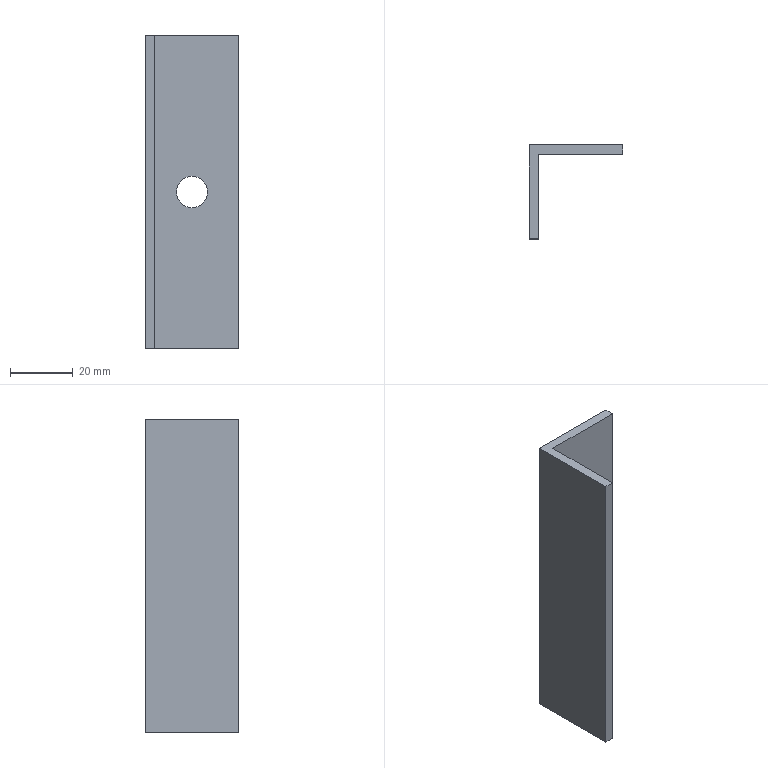Part | SolidWorks | features Extrusion 1, ICE 1 | 1 solid | 10 faces | box 30 x 30 x 100 mm | volume 16864 mm3 | plane 8 | cylinder 2 | commonest cylinder face diameters 10 x2
STEP:
#1=CARTESIAN_POINT('',(15.,-3.,45.));
#2=VERTEX_POINT('',#1);
#3=CARTESIAN_POINT('',(15.,-3.,55.));
#4=VERTEX_POINT('',#3);
#5=CARTESIAN_POINT('',(15.,-3.,50.));
#6=DIRECTION('',(0.,1.,0.));
#7=DIRECTION('',(0.,0.,1.));
#8=AXIS2_PLACEMENT_3D('',#5,#6,#7);
#9=CIRCLE('',#8,5.);
#10=EDGE_CURVE('',#2,#4,#9,.T.);
#11=ORIENTED_EDGE('',*,*,#10,.F.);
#12=CARTESIAN_POINT('',(15.,0.,45.));
#13=VERTEX_POINT('',#12);
#14=CARTESIAN_POINT('',(15.,-10.,45.));
#15=DIRECTION('',(0.,1.,0.));
#16=VECTOR('',#15,1000.);
#17=LINE('',#14,#16);
#18=EDGE_CURVE('',#2,#13,#17,.T.);
#19=ORIENTED_EDGE('',*,*,#18,.T.);
#20=CARTESIAN_POINT('',(15.,0.,55.));
#21=VERTEX_POINT('',#20);
#22=CARTESIAN_POINT('',(15.,0.,50.));
#23=DIRECTION('',(0.,1.,0.));
#24=DIRECTION('',(0.,0.,1.));
#25=AXIS2_PLACEMENT_3D('',#22,#23,#24);
#26=CIRCLE('',#25,5.);
#27=EDGE_CURVE('',#13,#21,#26,.T.);
#28=ORIENTED_EDGE('',*,*,#27,.T.);
#29=CARTESIAN_POINT('',(15.,-10.,55.));
#30=DIRECTION('',(0.,1.,0.));
#31=VECTOR('',#30,1000.);
#32=LINE('',#29,#31);
#33=EDGE_CURVE('',#4,#21,#32,.T.);
#34=ORIENTED_EDGE('',*,*,#33,.F.);
#35=EDGE_LOOP('',(#11,#19,#28,#34));
#36=FACE_OUTER_BOUND('',#35,.T.);
#37=CARTESIAN_POINT('',(15.,-10.,50.));
#38=DIRECTION('',(0.,1.,0.));
#39=DIRECTION('',(0.,0.,1.));
#40=AXIS2_PLACEMENT_3D('',#37,#38,#39);
#41=CYLINDRICAL_SURFACE('',#40,5.);
#42=ADVANCED_FACE('',(#36),#41,.F.);
#43=CARTESIAN_POINT('',(0.,0.,0.));
#44=VERTEX_POINT('',#43);
#45=CARTESIAN_POINT('',(0.,-30.,0.));
#46=VERTEX_POINT('',#45);
#47=CARTESIAN_POINT('',(0.,0.,0.));
#48=DIRECTION('',(0.,-1.,0.));
#49=VECTOR('',#48,1000.);
#50=LINE('',#47,#49);
#51=EDGE_CURVE('',#44,#46,#50,.T.);
#52=ORIENTED_EDGE('',*,*,#51,.T.);
#53=CARTESIAN_POINT('',(0.,-30.,100.));
#54=VERTEX_POINT('',#53);
#55=CARTESIAN_POINT('',(0.,-30.,100.));
#56=DIRECTION('',(0.,0.,-1.));
#57=VECTOR('',#56,1000.);
#58=LINE('',#55,#57);
#59=EDGE_CURVE('',#54,#46,#58,.T.);
#60=ORIENTED_EDGE('',*,*,#59,.F.);
#61=CARTESIAN_POINT('',(0.,0.,100.));
#62=VERTEX_POINT('',#61);
#63=CARTESIAN_POINT('',(0.,0.,100.));
#64=DIRECTION('',(0.,-1.,0.));
#65=VECTOR('',#64,1000.);
#66=LINE('',#63,#65);
#67=EDGE_CURVE('',#62,#54,#66,.T.);
#68=ORIENTED_EDGE('',*,*,#67,.F.);
#69=CARTESIAN_POINT('',(0.,0.,100.));
#70=DIRECTION('',(0.,0.,-1.));
#71=VECTOR('',#70,1000.);
#72=LINE('',#69,#71);
#73=EDGE_CURVE('',#62,#44,#72,.T.);
#74=ORIENTED_EDGE('',*,*,#73,.T.);
#75=EDGE_LOOP('',(#52,#60,#68,#74));
#76=FACE_OUTER_BOUND('',#75,.T.);
#77=CARTESIAN_POINT('',(0.,0.,100.));
#78=DIRECTION('',(1.,0.,0.));
#79=DIRECTION('',(0.,1.,0.));
#80=AXIS2_PLACEMENT_3D('',#77,#78,#79);
#81=PLANE('',#80);
#82=ADVANCED_FACE('',(#76),#81,.F.);
#83=CARTESIAN_POINT('',(3.,-30.,0.));
#84=VERTEX_POINT('',#83);
#85=CARTESIAN_POINT('',(0.,-30.,0.));
#86=DIRECTION('',(1.,0.,0.));
#87=VECTOR('',#86,1000.);
#88=LINE('',#85,#87);
#89=EDGE_CURVE('',#46,#84,#88,.T.);
#90=ORIENTED_EDGE('',*,*,#89,.T.);
#91=CARTESIAN_POINT('',(3.,-30.,100.));
#92=VERTEX_POINT('',#91);
#93=CARTESIAN_POINT('',(3.,-30.,100.));
#94=DIRECTION('',(0.,0.,-1.));
#95=VECTOR('',#94,1000.);
#96=LINE('',#93,#95);
#97=EDGE_CURVE('',#92,#84,#96,.T.);
#98=ORIENTED_EDGE('',*,*,#97,.F.);
#99=CARTESIAN_POINT('',(0.,-30.,100.));
#100=DIRECTION('',(1.,0.,0.));
#101=VECTOR('',#100,1000.);
#102=LINE('',#99,#101);
#103=EDGE_CURVE('',#54,#92,#102,.T.);
#104=ORIENTED_EDGE('',*,*,#103,.F.);
#105=ORIENTED_EDGE('',*,*,#59,.T.);
#106=EDGE_LOOP('',(#90,#98,#104,#105));
#107=FACE_OUTER_BOUND('',#106,.T.);
#108=CARTESIAN_POINT('',(0.,-30.,100.));
#109=DIRECTION('',(0.,1.,0.));
#110=DIRECTION('',(0.,0.,1.));
#111=AXIS2_PLACEMENT_3D('',#108,#109,#110);
#112=PLANE('',#111);
#113=ADVANCED_FACE('',(#107),#112,.F.);
#114=CARTESIAN_POINT('',(3.,-3.,0.));
#115=VERTEX_POINT('',#114);
#116=CARTESIAN_POINT('',(3.,-3.,0.));
#117=DIRECTION('',(0.,1.,0.));
#118=VECTOR('',#117,1000.);
#119=LINE('',#116,#118);
#120=EDGE_CURVE('',#84,#115,#119,.T.);
#121=ORIENTED_EDGE('',*,*,#120,.T.);
#122=CARTESIAN_POINT('',(3.,-3.,100.));
#123=VERTEX_POINT('',#122);
#124=CARTESIAN_POINT('',(3.,-3.,100.));
#125=DIRECTION('',(0.,0.,-1.));
#126=VECTOR('',#125,1000.);
#127=LINE('',#124,#126);
#128=EDGE_CURVE('',#123,#115,#127,.T.);
#129=ORIENTED_EDGE('',*,*,#128,.F.);
#130=CARTESIAN_POINT('',(3.,-3.,100.));
#131=DIRECTION('',(0.,1.,0.));
#132=VECTOR('',#131,1000.);
#133=LINE('',#130,#132);
#134=EDGE_CURVE('',#92,#123,#133,.T.);
#135=ORIENTED_EDGE('',*,*,#134,.F.);
#136=ORIENTED_EDGE('',*,*,#97,.T.);
#137=EDGE_LOOP('',(#121,#129,#135,#136));
#138=FACE_OUTER_BOUND('',#137,.T.);
#139=CARTESIAN_POINT('',(3.,-3.,100.));
#140=DIRECTION('',(-1.,0.,0.));
#141=DIRECTION('',(0.,0.,1.));
#142=AXIS2_PLACEMENT_3D('',#139,#140,#141);
#143=PLANE('',#142);
#144=ADVANCED_FACE('',(#138),#143,.F.);
#145=CARTESIAN_POINT('',(15.,-3.,50.));
#146=DIRECTION('',(0.,1.,0.));
#147=DIRECTION('',(0.,0.,1.));
#148=AXIS2_PLACEMENT_3D('',#145,#146,#147);
#149=CIRCLE('',#148,5.);
#150=EDGE_CURVE('',#4,#2,#149,.T.);
#151=ORIENTED_EDGE('',*,*,#150,.T.);
#152=ORIENTED_EDGE('',*,*,#10,.T.);
#153=EDGE_LOOP('',(#151,#152));
#154=FACE_BOUND('',#153,.T.);
#155=CARTESIAN_POINT('',(30.,-3.,0.));
#156=VERTEX_POINT('',#155);
#157=CARTESIAN_POINT('',(3.,-3.,0.));
#158=DIRECTION('',(1.,0.,0.));
#159=VECTOR('',#158,1000.);
#160=LINE('',#157,#159);
#161=EDGE_CURVE('',#115,#156,#160,.T.);
#162=ORIENTED_EDGE('',*,*,#161,.T.);
#163=CARTESIAN_POINT('',(30.,-3.,100.));
#164=VERTEX_POINT('',#163);
#165=CARTESIAN_POINT('',(30.,-3.,100.));
#166=DIRECTION('',(0.,0.,-1.));
#167=VECTOR('',#166,1000.);
#168=LINE('',#165,#167);
#169=EDGE_CURVE('',#164,#156,#168,.T.);
#170=ORIENTED_EDGE('',*,*,#169,.F.);
#171=CARTESIAN_POINT('',(3.,-3.,100.));
#172=DIRECTION('',(1.,0.,0.));
#173=VECTOR('',#172,1000.);
#174=LINE('',#171,#173);
#175=EDGE_CURVE('',#123,#164,#174,.T.);
#176=ORIENTED_EDGE('',*,*,#175,.F.);
#177=ORIENTED_EDGE('',*,*,#128,.T.);
#178=EDGE_LOOP('',(#162,#170,#176,#177));
#179=FACE_OUTER_BOUND('',#178,.T.);
#180=CARTESIAN_POINT('',(3.,-3.,100.));
#181=DIRECTION('',(0.,1.,0.));
#182=DIRECTION('',(0.,0.,1.));
#183=AXIS2_PLACEMENT_3D('',#180,#181,#182);
#184=PLANE('',#183);
#185=ADVANCED_FACE('',(#154,#179),#184,.F.);
#186=CARTESIAN_POINT('',(30.,0.,0.));
#187=VERTEX_POINT('',#186);
#188=CARTESIAN_POINT('',(30.,-3.,0.));
#189=DIRECTION('',(0.,1.,0.));
#190=VECTOR('',#189,1000.);
#191=LINE('',#188,#190);
#192=EDGE_CURVE('',#156,#187,#191,.T.);
#193=ORIENTED_EDGE('',*,*,#192,.T.);
#194=CARTESIAN_POINT('',(30.,0.,100.));
#195=VERTEX_POINT('',#194);
#196=CARTESIAN_POINT('',(30.,0.,100.));
#197=DIRECTION('',(0.,0.,-1.));
#198=VECTOR('',#197,1000.);
#199=LINE('',#196,#198);
#200=EDGE_CURVE('',#195,#187,#199,.T.);
#201=ORIENTED_EDGE('',*,*,#200,.F.);
#202=CARTESIAN_POINT('',(30.,-3.,100.));
#203=DIRECTION('',(0.,1.,0.));
#204=VECTOR('',#203,1000.);
#205=LINE('',#202,#204);
#206=EDGE_CURVE('',#164,#195,#205,.T.);
#207=ORIENTED_EDGE('',*,*,#206,.F.);
#208=ORIENTED_EDGE('',*,*,#169,.T.);
#209=EDGE_LOOP('',(#193,#201,#207,#208));
#210=FACE_OUTER_BOUND('',#209,.T.);
#211=CARTESIAN_POINT('',(30.,-3.,100.));
#212=DIRECTION('',(-1.,0.,0.));
#213=DIRECTION('',(0.,0.,1.));
#214=AXIS2_PLACEMENT_3D('',#211,#212,#213);
#215=PLANE('',#214);
#216=ADVANCED_FACE('',(#210),#215,.F.);
#217=CARTESIAN_POINT('',(15.,0.,50.));
#218=DIRECTION('',(0.,1.,0.));
#219=DIRECTION('',(0.,0.,1.));
#220=AXIS2_PLACEMENT_3D('',#217,#218,#219);
#221=CIRCLE('',#220,5.);
#222=EDGE_CURVE('',#21,#13,#221,.T.);
#223=ORIENTED_EDGE('',*,*,#222,.F.);
#224=ORIENTED_EDGE('',*,*,#27,.F.);
#225=EDGE_LOOP('',(#223,#224));
#226=FACE_BOUND('',#225,.T.);
#227=CARTESIAN_POINT('',(0.,0.,0.));
#228=DIRECTION('',(-1.,0.,0.));
#229=VECTOR('',#228,1000.);
#230=LINE('',#227,#229);
#231=EDGE_CURVE('',#187,#44,#230,.T.);
#232=ORIENTED_EDGE('',*,*,#231,.T.);
#233=ORIENTED_EDGE('',*,*,#73,.F.);
#234=CARTESIAN_POINT('',(0.,0.,100.));
#235=DIRECTION('',(-1.,0.,0.));
#236=VECTOR('',#235,1000.);
#237=LINE('',#234,#236);
#238=EDGE_CURVE('',#195,#62,#237,.T.);
#239=ORIENTED_EDGE('',*,*,#238,.F.);
#240=ORIENTED_EDGE('',*,*,#200,.T.);
#241=EDGE_LOOP('',(#232,#233,#239,#240));
#242=FACE_OUTER_BOUND('',#241,.T.);
#243=CARTESIAN_POINT('',(0.,0.,100.));
#244=DIRECTION('',(0.,-1.,0.));
#245=DIRECTION('',(0.,0.,-1.));
#246=AXIS2_PLACEMENT_3D('',#243,#244,#245);
#247=PLANE('',#246);
#248=ADVANCED_FACE('',(#226,#242),#247,.F.);
#249=ORIENTED_EDGE('',*,*,#67,.T.);
#250=ORIENTED_EDGE('',*,*,#103,.T.);
#251=ORIENTED_EDGE('',*,*,#134,.T.);
#252=ORIENTED_EDGE('',*,*,#175,.T.);
#253=ORIENTED_EDGE('',*,*,#206,.T.);
#254=ORIENTED_EDGE('',*,*,#238,.T.);
#255=EDGE_LOOP('',(#249,#250,#251,#252,#253,#254));
#256=FACE_OUTER_BOUND('',#255,.T.);
#257=CARTESIAN_POINT('',(0.,0.,100.));
#258=DIRECTION('',(0.,0.,1.));
#259=DIRECTION('',(1.,0.,0.));
#260=AXIS2_PLACEMENT_3D('',#257,#258,#259);
#261=PLANE('',#260);
#262=ADVANCED_FACE('',(#256),#261,.T.);
#263=ORIENTED_EDGE('',*,*,#51,.F.);
#264=ORIENTED_EDGE('',*,*,#231,.F.);
#265=ORIENTED_EDGE('',*,*,#192,.F.);
#266=ORIENTED_EDGE('',*,*,#161,.F.);
#267=ORIENTED_EDGE('',*,*,#120,.F.);
#268=ORIENTED_EDGE('',*,*,#89,.F.);
#269=EDGE_LOOP('',(#263,#264,#265,#266,#267,#268));
#270=FACE_OUTER_BOUND('',#269,.T.);
#271=CARTESIAN_POINT('',(0.,0.,0.));
#272=DIRECTION('',(0.,0.,1.));
#273=DIRECTION('',(1.,0.,0.));
#274=AXIS2_PLACEMENT_3D('',#271,#272,#273);
#275=PLANE('',#274);
#276=ADVANCED_FACE('',(#270),#275,.F.);
#277=ORIENTED_EDGE('',*,*,#18,.F.);
#278=ORIENTED_EDGE('',*,*,#150,.F.);
#279=ORIENTED_EDGE('',*,*,#33,.T.);
#280=ORIENTED_EDGE('',*,*,#222,.T.);
#281=EDGE_LOOP('',(#277,#278,#279,#280));
#282=FACE_OUTER_BOUND('',#281,.T.);
#283=CARTESIAN_POINT('',(15.,-10.,50.));
#284=DIRECTION('',(0.,1.,0.));
#285=DIRECTION('',(0.,0.,1.));
#286=AXIS2_PLACEMENT_3D('',#283,#284,#285);
#287=CYLINDRICAL_SURFACE('',#286,5.);
#288=ADVANCED_FACE('',(#282),#287,.F.);
#289=CLOSED_SHELL('',(#42,#82,#113,#144,#185,#216,#248,#262,#276,#288));
#290=MANIFOLD_SOLID_BREP('',#289);
#291=CARTESIAN_POINT('',(0.,0.,0.));
#292=DIRECTION('',(0.,0.,1.));
#293=DIRECTION('',(1.,0.,0.));
#294=AXIS2_PLACEMENT_3D('',#291,#292,#293);
#295=(LENGTH_UNIT()NAMED_UNIT(*)SI_UNIT(.MILLI.,.METRE.));
#296=UNCERTAINTY_MEASURE_WITH_UNIT(LENGTH_MEASURE(0.00001),#295,'','');
#297=(NAMED_UNIT(*)PLANE_ANGLE_UNIT()SI_UNIT($,.RADIAN.));
#298=(NAMED_UNIT(*)SI_UNIT($,.STERADIAN.)SOLID_ANGLE_UNIT());
#299=(GEOMETRIC_REPRESENTATION_CONTEXT(3)GLOBAL_UNCERTAINTY_ASSIGNED_CONTEXT((#296))GLOBAL_UNIT_ASSIGNED_CONTEXT((#295,#297,#298))REPRESENTATION_CONTEXT('',''));
#300=ADVANCED_BREP_SHAPE_REPRESENTATION('',(#290,#294),#299);